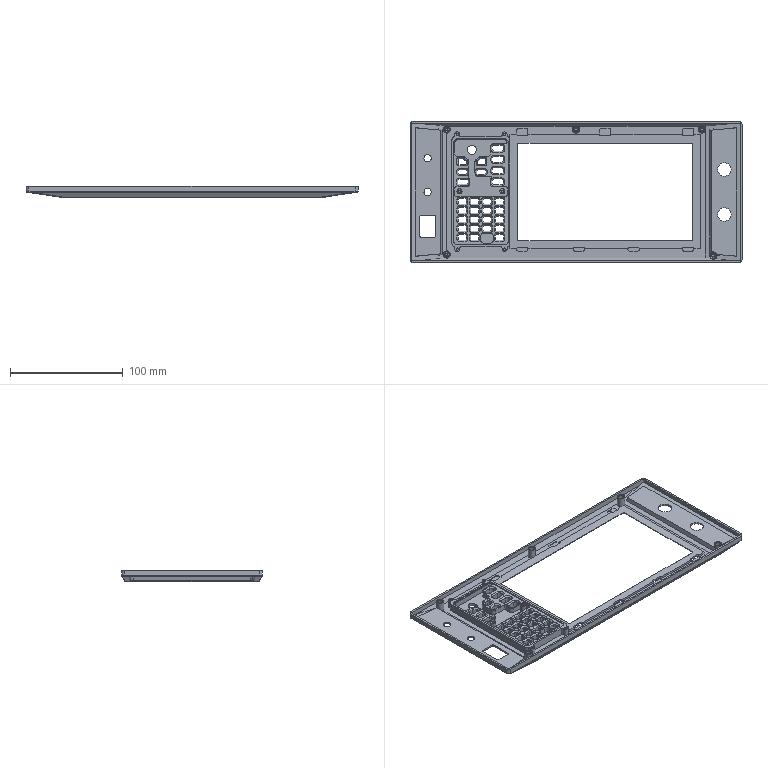NC program | NX | posted with a generic post | part box 295 x 125 x 10 mm
Lines 1 to 74 of 134431:
N10 G17 G21 G94 G90
(FLOOR_WALL , TOOL : D63)
N12 T01 M6
N14 G54
N16 G17 G0 G90 X-185. Y65.497 S6500 M3
N18 G43 Z30. H1
N20 Z3.
N22 G94 G1 Z0. F1250.
N24 X-182.
N26 X182.
N28 Y30.231
N30 X-182.
N32 Y-5.034
N34 X182.
N36 Y-40.3
N38 X-182.
N40 X-185.
N42 Z3.
N44 G0 Z30.
N46 M5
(DRILLING , TOOL : D6A45)
N48 T07 M6
N50 G54
N52 G17 G0 G90 X122. Y-56.5 S5000 M3
N54 G43 Z30. H7
N56 G94 G81 G98 Z-1. F250. R3.
N58 X0. Y55.5
N60 X-63.5 Y51.2
N62 X-105.5
N64 X-115. Y55.5
N66 X-103.5 Y0.59
N68 X-65.5
N70 X-63.5 Y-50.77
N72 X-105.5
N74 X-115. Y-55.5
N76 G80
N78 G0 X-115. Y-55.5 Z30.
N80 M5
(DRILLING_COPY , TOOL : 2.5ZT)
N82 T12 M6
N84 G54
N86 G17 G0 G90 X-115. Y55.5 S2000 M3
N88 G43 Z30. H12
N90 G94 G83 G98 Z-7.5 F120. Q2. R3.
N92 Y-55.5
N94 X112. Y55.5
N96 X122. Y-56.5
N98 G80
N100 G0 X122. Y-56.5 Z30.
N102 M5
(DRILLING_COPY_COPY , TOOL : 2.1ZT)
N104 T13 M6
N106 G54
N108 G17 G0 G90 X-63.5 Y-50.77 S2000 M3
N110 G43 Z30. H13
N112 G94 G83 G98 Z-7.5 F120. Q2. R3.
N114 X-105.5
N116 X-103.5 Y0.59
N118 X-65.5
N120 X-63.5 Y51.2
N122 X-105.5
N124 G80
N126 G0 X-105.5 Y51.2 Z30.
N128 M5